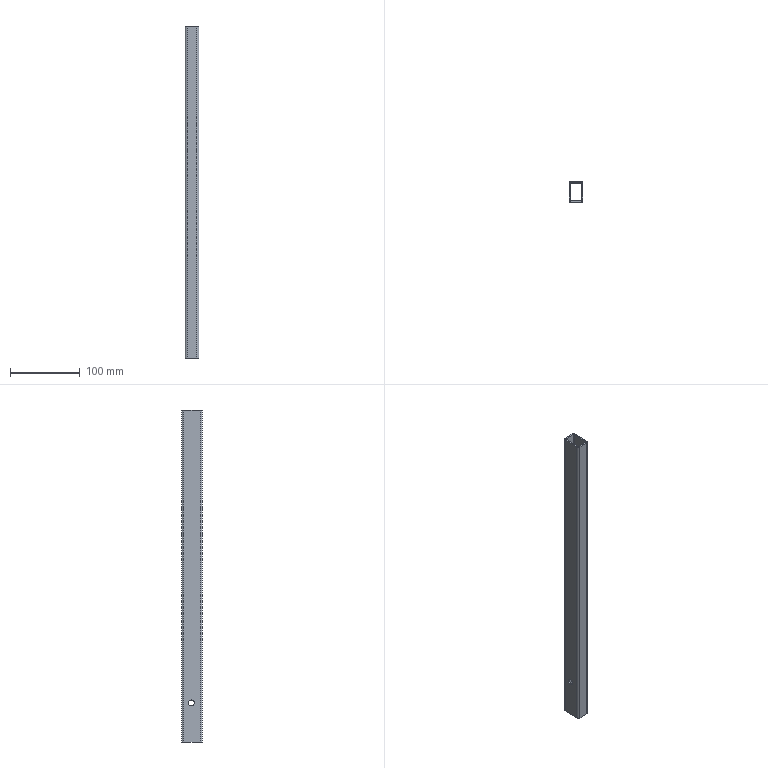Part | STEP file | DIN EN 10305-5 - 35 x 20 x 2  - 454 | 1 solid | 20 faces | box 20 x 30 x 475 mm | volume 83922 mm3 | cylinder 10 | plane 10 | commonest cylinder face diameters 2 x4 6 x4 8.3 x2